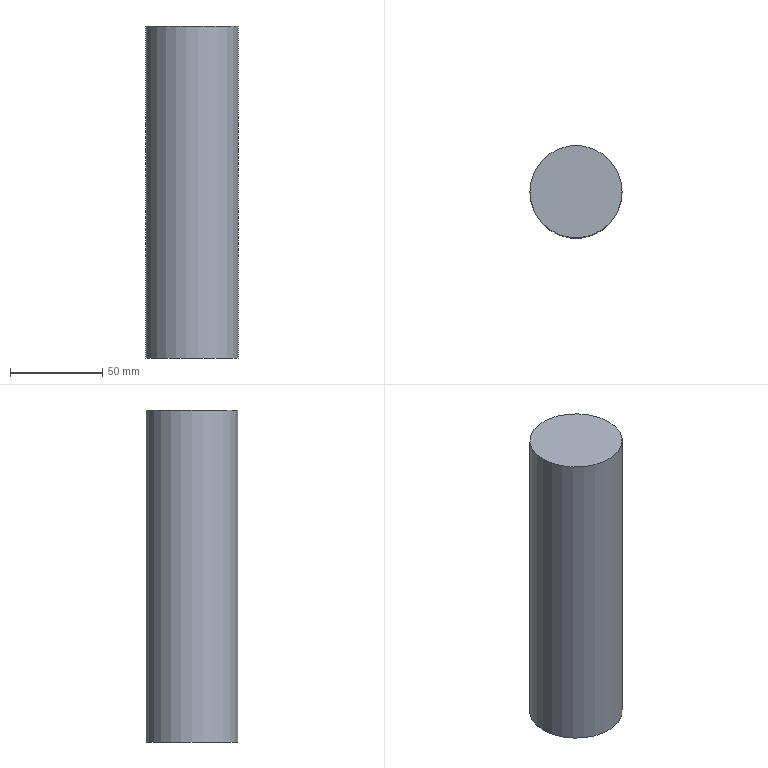Part | NX | features solid 2 | 1 solid | 3 faces | box 50 x 50 x 180 mm | volume 353429 mm3 | plane 2 | cylinder 1 | commonest cylinder face diameters 50 x1
STEP:
#1=CARTESIAN_POINT('',(970.,395.,2.));
#2=VERTEX_POINT('',#1);
#3=CARTESIAN_POINT('',(995.,395.,2.));
#4=DIRECTION('',(0.,0.,-1.));
#5=DIRECTION('',(-1.,0.,0.));
#6=AXIS2_PLACEMENT_3D('',#3,#4,#5);
#7=CIRCLE('',#6,25.);
#8=EDGE_CURVE('',#2,#2,#7,.F.);
#9=ORIENTED_EDGE('',*,*,#8,.F.);
#10=EDGE_LOOP('',(#9));
#11=FACE_BOUND('',#10,.T.);
#12=CARTESIAN_POINT('',(1020.,395.,-178.));
#13=VERTEX_POINT('',#12);
#14=CARTESIAN_POINT('',(995.,395.,-178.));
#15=DIRECTION('',(0.,0.,1.));
#16=DIRECTION('',(1.,0.,0.));
#17=AXIS2_PLACEMENT_3D('',#14,#15,#16);
#18=CIRCLE('',#17,25.);
#19=EDGE_CURVE('',#13,#13,#18,.F.);
#20=ORIENTED_EDGE('',*,*,#19,.F.);
#21=EDGE_LOOP('',(#20));
#22=FACE_BOUND('',#21,.T.);
#23=CARTESIAN_POINT('',(995.,395.,117.));
#24=DIRECTION('',(0.,0.,-1.));
#25=DIRECTION('',(1.,0.,0.));
#26=AXIS2_PLACEMENT_3D('',#23,#24,#25);
#27=CYLINDRICAL_SURFACE('',#26,25.);
#28=ADVANCED_FACE('',(#11,#22),#27,.T.);
#29=ORIENTED_EDGE('',*,*,#19,.T.);
#30=EDGE_LOOP('',(#29));
#31=FACE_BOUND('',#30,.T.);
#32=CARTESIAN_POINT('',(995.,395.,-178.));
#33=DIRECTION('',(0.,0.,1.));
#34=DIRECTION('',(-1.,0.,0.));
#35=AXIS2_PLACEMENT_3D('',#32,#33,#34);
#36=PLANE('',#35);
#37=ADVANCED_FACE('',(#31),#36,.F.);
#38=ORIENTED_EDGE('',*,*,#8,.T.);
#39=EDGE_LOOP('',(#38));
#40=FACE_BOUND('',#39,.T.);
#41=CARTESIAN_POINT('',(995.,395.,2.));
#42=DIRECTION('',(0.,0.,-1.));
#43=DIRECTION('',(1.,0.,0.));
#44=AXIS2_PLACEMENT_3D('',#41,#42,#43);
#45=PLANE('',#44);
#46=ADVANCED_FACE('',(#40),#45,.F.);
#47=CLOSED_SHELL('',(#28,#37,#46));
#48=MANIFOLD_SOLID_BREP('',#47);
#49=(LENGTH_UNIT()NAMED_UNIT(*)SI_UNIT(.MILLI.,.METRE.));
#50=UNCERTAINTY_MEASURE_WITH_UNIT(LENGTH_MEASURE(0.00001),#49,'','');
#51=(NAMED_UNIT(*)PLANE_ANGLE_UNIT()SI_UNIT($,.RADIAN.));
#52=(NAMED_UNIT(*)SI_UNIT($,.STERADIAN.)SOLID_ANGLE_UNIT());
#53=(GEOMETRIC_REPRESENTATION_CONTEXT(3)GLOBAL_UNCERTAINTY_ASSIGNED_CONTEXT((#50))GLOBAL_UNIT_ASSIGNED_CONTEXT((#49,#51,#52))REPRESENTATION_CONTEXT('',''));
#54=ADVANCED_BREP_SHAPE_REPRESENTATION('',(#48),#53);